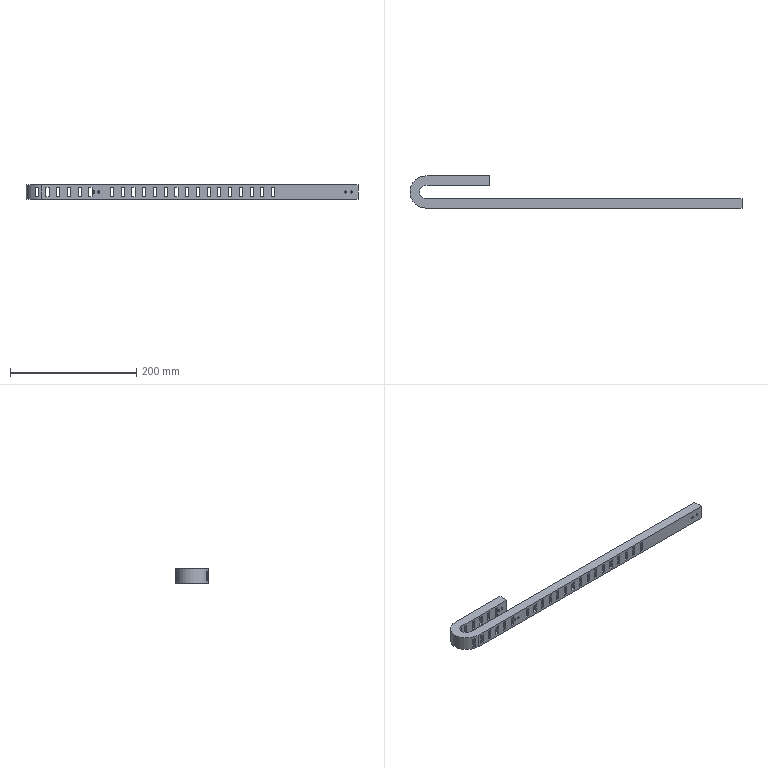Part | NX | 1 solid | 125 faces | box 525.5 x 51 x 22.5 mm | volume 188727 mm3 | plane 117 | cylinder 8 | commonest cylinder face diameters 3.5 x6 21 x1 51 x1